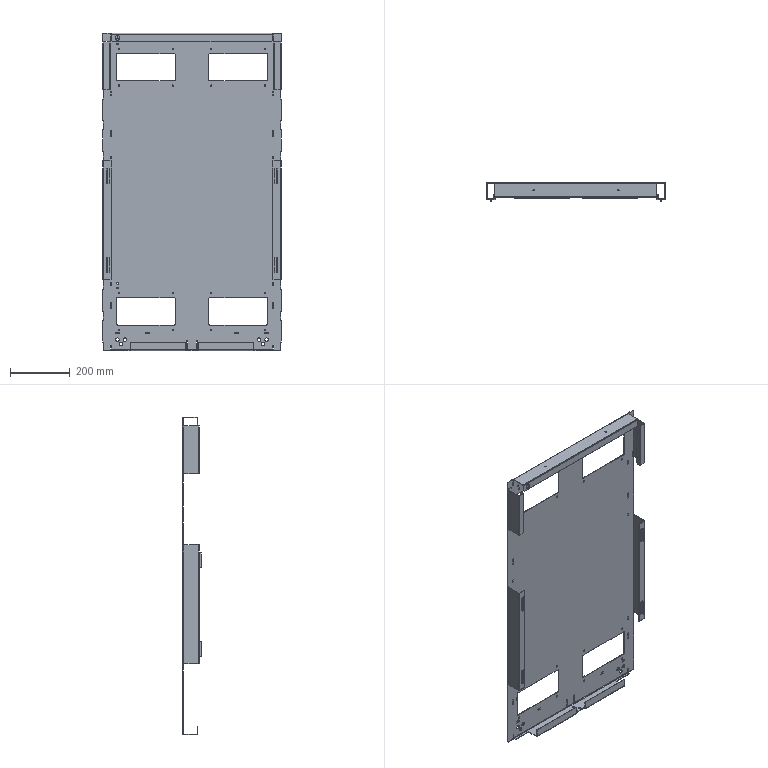Part | NX | features solid 2 | 1 solid | 610 faces | box 600 x 62.008 x 1068 mm | volume 1447139 mm3 | plane 418 | cylinder 159 | cone 32 | spline 1 | commonest cylinder face diameters 4.25 x32 4 x16 8 x16 2.5 x15 6.5 x15 5.64 x14